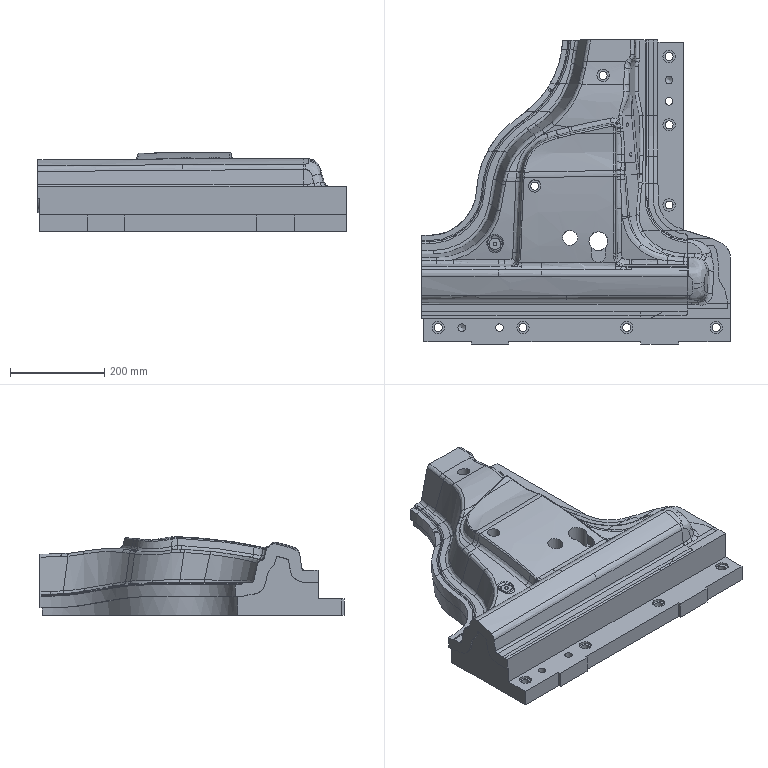Part | NX | features solid 2 | 1 solid | 452 faces | box 655 x 645 x 167.425 mm | volume 22826307 mm3 | spline 384 | plane 41 | cylinder 25 | cone 2 | commonest cylinder face diameters 17 x9 26 x9 16 x4 30 x1 32 x1 40 x1